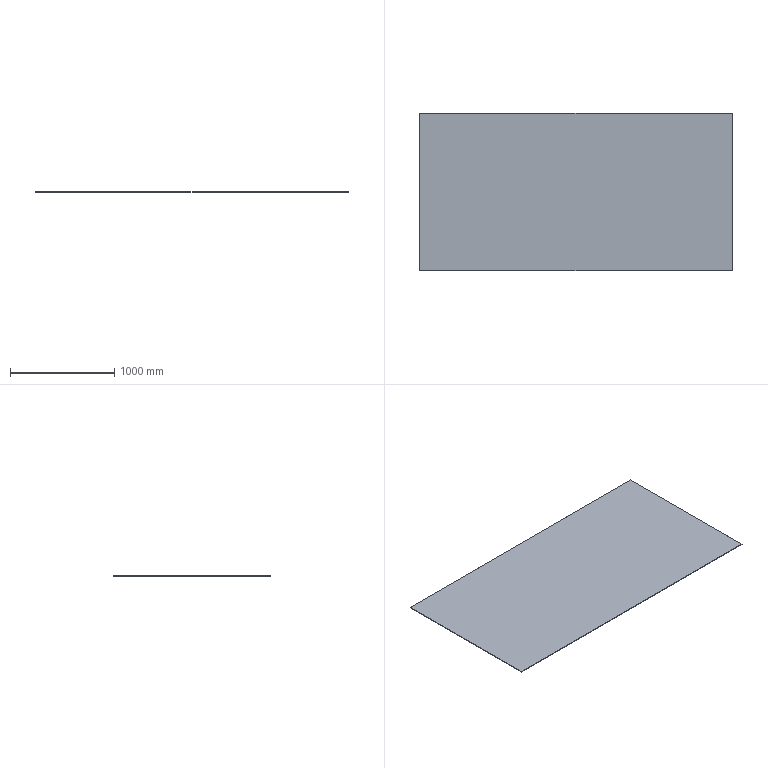Part | SolidWorks | features Extrusion 1 | 1 solid | 6 faces | box 3000 x 1510 x 6 mm | volume 27180000 mm3 | plane 6
STEP:
#1=CARTESIAN_POINT('',(0.,1510.,0.));
#2=VERTEX_POINT('',#1);
#3=CARTESIAN_POINT('',(0.,0.,0.));
#4=VERTEX_POINT('',#3);
#5=CARTESIAN_POINT('',(0.,0.,0.));
#6=DIRECTION('',(0.,-1.,0.));
#7=VECTOR('',#6,1000.);
#8=LINE('',#5,#7);
#9=EDGE_CURVE('',#2,#4,#8,.T.);
#10=ORIENTED_EDGE('',*,*,#9,.T.);
#11=CARTESIAN_POINT('',(0.,0.,6.));
#12=VERTEX_POINT('',#11);
#13=CARTESIAN_POINT('',(0.,0.,6.));
#14=DIRECTION('',(0.,0.,-1.));
#15=VECTOR('',#14,1000.);
#16=LINE('',#13,#15);
#17=EDGE_CURVE('',#12,#4,#16,.T.);
#18=ORIENTED_EDGE('',*,*,#17,.F.);
#19=CARTESIAN_POINT('',(0.,1510.,6.));
#20=VERTEX_POINT('',#19);
#21=CARTESIAN_POINT('',(0.,0.,6.));
#22=DIRECTION('',(0.,-1.,0.));
#23=VECTOR('',#22,1000.);
#24=LINE('',#21,#23);
#25=EDGE_CURVE('',#20,#12,#24,.T.);
#26=ORIENTED_EDGE('',*,*,#25,.F.);
#27=CARTESIAN_POINT('',(0.,1510.,6.));
#28=DIRECTION('',(0.,0.,-1.));
#29=VECTOR('',#28,1000.);
#30=LINE('',#27,#29);
#31=EDGE_CURVE('',#20,#2,#30,.T.);
#32=ORIENTED_EDGE('',*,*,#31,.T.);
#33=EDGE_LOOP('',(#10,#18,#26,#32));
#34=FACE_OUTER_BOUND('',#33,.T.);
#35=CARTESIAN_POINT('',(0.,0.,6.));
#36=DIRECTION('',(1.,0.,0.));
#37=DIRECTION('',(0.,0.,-1.));
#38=AXIS2_PLACEMENT_3D('',#35,#36,#37);
#39=PLANE('',#38);
#40=ADVANCED_FACE('',(#34),#39,.F.);
#41=CARTESIAN_POINT('',(3000.,0.,0.));
#42=VERTEX_POINT('',#41);
#43=CARTESIAN_POINT('',(0.,0.,0.));
#44=DIRECTION('',(1.,0.,0.));
#45=VECTOR('',#44,1000.);
#46=LINE('',#43,#45);
#47=EDGE_CURVE('',#4,#42,#46,.T.);
#48=ORIENTED_EDGE('',*,*,#47,.T.);
#49=CARTESIAN_POINT('',(3000.,0.,6.));
#50=VERTEX_POINT('',#49);
#51=CARTESIAN_POINT('',(3000.,0.,6.));
#52=DIRECTION('',(0.,0.,-1.));
#53=VECTOR('',#52,1000.);
#54=LINE('',#51,#53);
#55=EDGE_CURVE('',#50,#42,#54,.T.);
#56=ORIENTED_EDGE('',*,*,#55,.F.);
#57=CARTESIAN_POINT('',(0.,0.,6.));
#58=DIRECTION('',(1.,0.,0.));
#59=VECTOR('',#58,1000.);
#60=LINE('',#57,#59);
#61=EDGE_CURVE('',#12,#50,#60,.T.);
#62=ORIENTED_EDGE('',*,*,#61,.F.);
#63=ORIENTED_EDGE('',*,*,#17,.T.);
#64=EDGE_LOOP('',(#48,#56,#62,#63));
#65=FACE_OUTER_BOUND('',#64,.T.);
#66=CARTESIAN_POINT('',(0.,0.,6.));
#67=DIRECTION('',(0.,1.,0.));
#68=DIRECTION('',(0.,0.,1.));
#69=AXIS2_PLACEMENT_3D('',#66,#67,#68);
#70=PLANE('',#69);
#71=ADVANCED_FACE('',(#65),#70,.F.);
#72=CARTESIAN_POINT('',(3000.,1510.,0.));
#73=VERTEX_POINT('',#72);
#74=CARTESIAN_POINT('',(3000.,0.,0.));
#75=DIRECTION('',(0.,1.,0.));
#76=VECTOR('',#75,1000.);
#77=LINE('',#74,#76);
#78=EDGE_CURVE('',#42,#73,#77,.T.);
#79=ORIENTED_EDGE('',*,*,#78,.T.);
#80=CARTESIAN_POINT('',(3000.,1510.,6.));
#81=VERTEX_POINT('',#80);
#82=CARTESIAN_POINT('',(3000.,1510.,6.));
#83=DIRECTION('',(0.,0.,-1.));
#84=VECTOR('',#83,1000.);
#85=LINE('',#82,#84);
#86=EDGE_CURVE('',#81,#73,#85,.T.);
#87=ORIENTED_EDGE('',*,*,#86,.F.);
#88=CARTESIAN_POINT('',(3000.,0.,6.));
#89=DIRECTION('',(0.,1.,0.));
#90=VECTOR('',#89,1000.);
#91=LINE('',#88,#90);
#92=EDGE_CURVE('',#50,#81,#91,.T.);
#93=ORIENTED_EDGE('',*,*,#92,.F.);
#94=ORIENTED_EDGE('',*,*,#55,.T.);
#95=EDGE_LOOP('',(#79,#87,#93,#94));
#96=FACE_OUTER_BOUND('',#95,.T.);
#97=CARTESIAN_POINT('',(3000.,0.,6.));
#98=DIRECTION('',(-1.,0.,0.));
#99=DIRECTION('',(0.,0.,1.));
#100=AXIS2_PLACEMENT_3D('',#97,#98,#99);
#101=PLANE('',#100);
#102=ADVANCED_FACE('',(#96),#101,.F.);
#103=CARTESIAN_POINT('',(0.,1510.,0.));
#104=DIRECTION('',(-1.,0.,0.));
#105=VECTOR('',#104,1000.);
#106=LINE('',#103,#105);
#107=EDGE_CURVE('',#73,#2,#106,.T.);
#108=ORIENTED_EDGE('',*,*,#107,.T.);
#109=ORIENTED_EDGE('',*,*,#31,.F.);
#110=CARTESIAN_POINT('',(0.,1510.,6.));
#111=DIRECTION('',(-1.,0.,0.));
#112=VECTOR('',#111,1000.);
#113=LINE('',#110,#112);
#114=EDGE_CURVE('',#81,#20,#113,.T.);
#115=ORIENTED_EDGE('',*,*,#114,.F.);
#116=ORIENTED_EDGE('',*,*,#86,.T.);
#117=EDGE_LOOP('',(#108,#109,#115,#116));
#118=FACE_OUTER_BOUND('',#117,.T.);
#119=CARTESIAN_POINT('',(0.,1510.,6.));
#120=DIRECTION('',(0.,-1.,0.));
#121=DIRECTION('',(0.,0.,-1.));
#122=AXIS2_PLACEMENT_3D('',#119,#120,#121);
#123=PLANE('',#122);
#124=ADVANCED_FACE('',(#118),#123,.F.);
#125=ORIENTED_EDGE('',*,*,#25,.T.);
#126=ORIENTED_EDGE('',*,*,#61,.T.);
#127=ORIENTED_EDGE('',*,*,#92,.T.);
#128=ORIENTED_EDGE('',*,*,#114,.T.);
#129=EDGE_LOOP('',(#125,#126,#127,#128));
#130=FACE_OUTER_BOUND('',#129,.T.);
#131=CARTESIAN_POINT('',(0.,0.,6.));
#132=DIRECTION('',(0.,0.,-1.));
#133=DIRECTION('',(-1.,0.,0.));
#134=AXIS2_PLACEMENT_3D('',#131,#132,#133);
#135=PLANE('',#134);
#136=ADVANCED_FACE('',(#130),#135,.F.);
#137=ORIENTED_EDGE('',*,*,#9,.F.);
#138=ORIENTED_EDGE('',*,*,#107,.F.);
#139=ORIENTED_EDGE('',*,*,#78,.F.);
#140=ORIENTED_EDGE('',*,*,#47,.F.);
#141=EDGE_LOOP('',(#137,#138,#139,#140));
#142=FACE_OUTER_BOUND('',#141,.T.);
#143=CARTESIAN_POINT('',(0.,0.,0.));
#144=DIRECTION('',(0.,0.,-1.));
#145=DIRECTION('',(-1.,0.,0.));
#146=AXIS2_PLACEMENT_3D('',#143,#144,#145);
#147=PLANE('',#146);
#148=ADVANCED_FACE('',(#142),#147,.T.);
#149=CLOSED_SHELL('',(#40,#71,#102,#124,#136,#148));
#150=MANIFOLD_SOLID_BREP('',#149);
#151=CARTESIAN_POINT('',(0.,0.,0.));
#152=DIRECTION('',(0.,0.,1.));
#153=DIRECTION('',(1.,0.,0.));
#154=AXIS2_PLACEMENT_3D('',#151,#152,#153);
#155=(LENGTH_UNIT()NAMED_UNIT(*)SI_UNIT(.MILLI.,.METRE.));
#156=UNCERTAINTY_MEASURE_WITH_UNIT(LENGTH_MEASURE(0.00001),#155,'','');
#157=(NAMED_UNIT(*)PLANE_ANGLE_UNIT()SI_UNIT($,.RADIAN.));
#158=(NAMED_UNIT(*)SI_UNIT($,.STERADIAN.)SOLID_ANGLE_UNIT());
#159=(GEOMETRIC_REPRESENTATION_CONTEXT(3)GLOBAL_UNCERTAINTY_ASSIGNED_CONTEXT((#156))GLOBAL_UNIT_ASSIGNED_CONTEXT((#155,#157,#158))REPRESENTATION_CONTEXT('',''));
#160=ADVANCED_BREP_SHAPE_REPRESENTATION('',(#150,#154),#159);